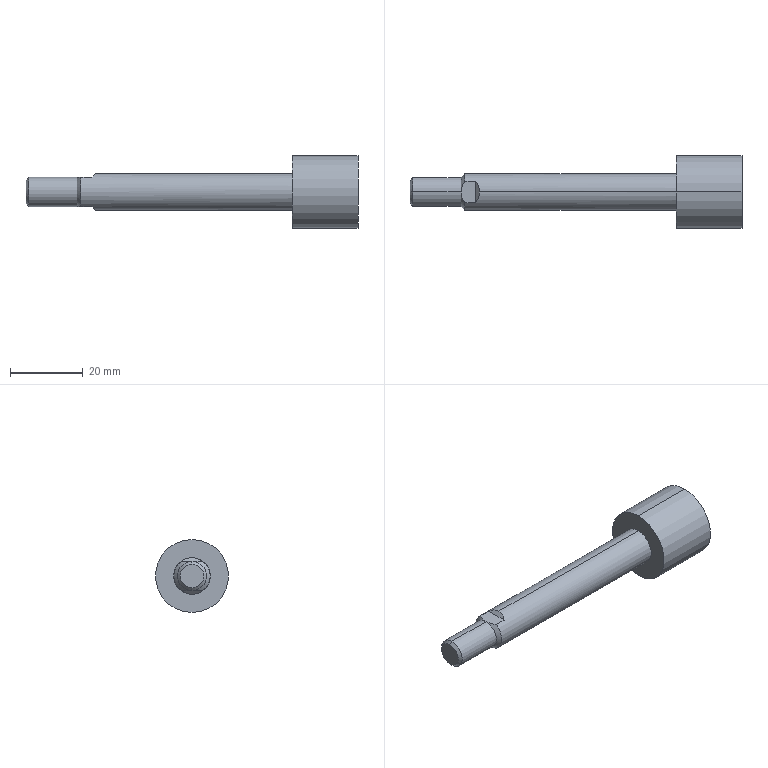Part | SolidWorks | features BaseBody 1 | 1 solid | 17 faces | box 91 x 20 x 20 mm | volume 10940 mm3 | plane 7 | cylinder 6 | cone 4 | commonest cylinder face diameters 8 x2 10 x2 20 x2
STEP:
#1=CARTESIAN_POINT('',(0.5,0.,5.));
#2=VERTEX_POINT('',#1);
#3=CARTESIAN_POINT('',(-0.5,3.,4.));
#4=VERTEX_POINT('',#3);
#5=CARTESIAN_POINT('',(0.5,0.,5.));
#6=CARTESIAN_POINT('',(0.5,1.091,5.));
#7=CARTESIAN_POINT('',(0.1549,2.127,4.655));
#8=CARTESIAN_POINT('',(-0.5,3.,4.));
#9=(BOUNDED_CURVE()B_SPLINE_CURVE(3,(#5,#6,#7,#8),.UNSPECIFIED.,.F.,.F.)B_SPLINE_CURVE_WITH_KNOTS((4,4),(0.,0.6435),.UNSPECIFIED.)CURVE()GEOMETRIC_REPRESENTATION_ITEM()RATIONAL_B_SPLINE_CURVE((1.,0.9658,0.9658,1.))REPRESENTATION_ITEM(''));
#10=EDGE_CURVE('',#2,#4,#9,.T.);
#11=ORIENTED_EDGE('',*,*,#10,.F.);
#12=CARTESIAN_POINT('',(54.5,0.,5.));
#13=VERTEX_POINT('',#12);
#14=CARTESIAN_POINT('',(72.5,0.,5.));
#15=DIRECTION('',(1.,0.,0.));
#16=VECTOR('',#15,1000.);
#17=LINE('',#14,#16);
#18=EDGE_CURVE('',#2,#13,#17,.T.);
#19=ORIENTED_EDGE('',*,*,#18,.T.);
#20=CARTESIAN_POINT('',(54.5,0.,-5.));
#21=VERTEX_POINT('',#20);
#22=CARTESIAN_POINT('',(54.5,0.,0.));
#23=DIRECTION('',(1.,0.,0.));
#24=DIRECTION('',(0.,0.,-1.));
#25=AXIS2_PLACEMENT_3D('',#22,#23,#24);
#26=CIRCLE('',#25,5.);
#27=EDGE_CURVE('',#21,#13,#26,.T.);
#28=ORIENTED_EDGE('',*,*,#27,.F.);
#29=CARTESIAN_POINT('',(0.5,0.,-5.));
#30=VERTEX_POINT('',#29);
#31=CARTESIAN_POINT('',(72.5,0.,-5.));
#32=DIRECTION('',(1.,0.,0.));
#33=VECTOR('',#32,1000.);
#34=LINE('',#31,#33);
#35=EDGE_CURVE('',#30,#21,#34,.T.);
#36=ORIENTED_EDGE('',*,*,#35,.F.);
#37=CARTESIAN_POINT('',(-0.5,3.,-4.));
#38=VERTEX_POINT('',#37);
#39=CARTESIAN_POINT('',(-0.5,3.,-4.));
#40=CARTESIAN_POINT('',(0.1549,2.127,-4.655));
#41=CARTESIAN_POINT('',(0.5,1.091,-5.));
#42=CARTESIAN_POINT('',(0.5,0.,-5.));
#43=(BOUNDED_CURVE()B_SPLINE_CURVE(3,(#39,#40,#41,#42),.UNSPECIFIED.,.F.,.T.)B_SPLINE_CURVE_WITH_KNOTS((4,4),(5.64,6.283),.UNSPECIFIED.)CURVE()GEOMETRIC_REPRESENTATION_ITEM()RATIONAL_B_SPLINE_CURVE((1.,0.9658,0.9658,1.))REPRESENTATION_ITEM(''));
#44=EDGE_CURVE('',#38,#30,#43,.T.);
#45=ORIENTED_EDGE('',*,*,#44,.F.);
#46=CARTESIAN_POINT('',(-3.5,3.,-4.));
#47=VERTEX_POINT('',#46);
#48=CARTESIAN_POINT('',(72.5,3.,-4.));
#49=DIRECTION('',(1.,0.,0.));
#50=VECTOR('',#49,1000.);
#51=LINE('',#48,#50);
#52=EDGE_CURVE('',#47,#38,#51,.T.);
#53=ORIENTED_EDGE('',*,*,#52,.F.);
#54=CARTESIAN_POINT('',(-3.5,3.,4.));
#55=VERTEX_POINT('',#54);
#56=CARTESIAN_POINT('',(-3.5,0.,0.));
#57=DIRECTION('',(1.,0.,0.));
#58=DIRECTION('',(0.,0.,-1.));
#59=AXIS2_PLACEMENT_3D('',#56,#57,#58);
#60=CIRCLE('',#59,5.);
#61=EDGE_CURVE('',#47,#55,#60,.T.);
#62=ORIENTED_EDGE('',*,*,#61,.T.);
#63=CARTESIAN_POINT('',(72.5,3.,4.));
#64=DIRECTION('',(-1.,0.,0.));
#65=VECTOR('',#64,1000.);
#66=LINE('',#63,#65);
#67=EDGE_CURVE('',#4,#55,#66,.T.);
#68=ORIENTED_EDGE('',*,*,#67,.F.);
#69=EDGE_LOOP('',(#11,#19,#28,#36,#45,#53,#62,#68));
#70=FACE_OUTER_BOUND('',#69,.T.);
#71=CARTESIAN_POINT('',(72.5,0.,0.));
#72=DIRECTION('',(1.,0.,0.));
#73=DIRECTION('',(0.,0.,-1.));
#74=AXIS2_PLACEMENT_3D('',#71,#72,#73);
#75=CYLINDRICAL_SURFACE('',#74,5.);
#76=ADVANCED_FACE('',(#70),#75,.T.);
#77=CARTESIAN_POINT('',(54.5,0.,-10.));
#78=VERTEX_POINT('',#77);
#79=CARTESIAN_POINT('',(54.5,0.,10.));
#80=VERTEX_POINT('',#79);
#81=CARTESIAN_POINT('',(54.5,0.,0.));
#82=DIRECTION('',(1.,0.,0.));
#83=DIRECTION('',(0.,0.,-1.));
#84=AXIS2_PLACEMENT_3D('',#81,#82,#83);
#85=CIRCLE('',#84,10.);
#86=EDGE_CURVE('',#78,#80,#85,.T.);
#87=ORIENTED_EDGE('',*,*,#86,.T.);
#88=CARTESIAN_POINT('',(72.5,0.,10.));
#89=VERTEX_POINT('',#88);
#90=CARTESIAN_POINT('',(72.5,0.,10.));
#91=DIRECTION('',(1.,0.,0.));
#92=VECTOR('',#91,1000.);
#93=LINE('',#90,#92);
#94=EDGE_CURVE('',#80,#89,#93,.T.);
#95=ORIENTED_EDGE('',*,*,#94,.T.);
#96=CARTESIAN_POINT('',(72.5,0.,-10.));
#97=VERTEX_POINT('',#96);
#98=CARTESIAN_POINT('',(72.5,0.,0.));
#99=DIRECTION('',(1.,0.,0.));
#100=DIRECTION('',(0.,0.,-1.));
#101=AXIS2_PLACEMENT_3D('',#98,#99,#100);
#102=CIRCLE('',#101,10.);
#103=EDGE_CURVE('',#97,#89,#102,.T.);
#104=ORIENTED_EDGE('',*,*,#103,.F.);
#105=CARTESIAN_POINT('',(72.5,0.,-10.));
#106=DIRECTION('',(1.,0.,0.));
#107=VECTOR('',#106,1000.);
#108=LINE('',#105,#107);
#109=EDGE_CURVE('',#78,#97,#108,.T.);
#110=ORIENTED_EDGE('',*,*,#109,.F.);
#111=EDGE_LOOP('',(#87,#95,#104,#110));
#112=FACE_OUTER_BOUND('',#111,.T.);
#113=CARTESIAN_POINT('',(72.5,0.,0.));
#114=DIRECTION('',(1.,0.,0.));
#115=DIRECTION('',(0.,0.,-1.));
#116=AXIS2_PLACEMENT_3D('',#113,#114,#115);
#117=CYLINDRICAL_SURFACE('',#116,10.);
#118=ADVANCED_FACE('',(#112),#117,.T.);
#119=CARTESIAN_POINT('',(-18.5,0.,-3.233));
#120=VERTEX_POINT('',#119);
#121=CARTESIAN_POINT('',(-18.5,0.,3.233));
#122=VERTEX_POINT('',#121);
#123=CARTESIAN_POINT('',(-18.5,0.,0.));
#124=DIRECTION('',(1.,0.,0.));
#125=DIRECTION('',(0.,0.,-1.));
#126=AXIS2_PLACEMENT_3D('',#123,#124,#125);
#127=CIRCLE('',#126,3.233);
#128=EDGE_CURVE('',#120,#122,#127,.T.);
#129=ORIENTED_EDGE('',*,*,#128,.T.);
#130=CARTESIAN_POINT('',(-17.733,0.,4.));
#131=VERTEX_POINT('',#130);
#132=CARTESIAN_POINT('',(-18.5,0.,3.233));
#133=DIRECTION('',(0.7071,0.,0.7071));
#134=VECTOR('',#133,1000.);
#135=LINE('',#132,#134);
#136=EDGE_CURVE('',#122,#131,#135,.T.);
#137=ORIENTED_EDGE('',*,*,#136,.T.);
#138=CARTESIAN_POINT('',(-17.733,0.,-4.));
#139=VERTEX_POINT('',#138);
#140=CARTESIAN_POINT('',(-17.733,0.,0.));
#141=DIRECTION('',(1.,0.,0.));
#142=DIRECTION('',(0.,0.,-1.));
#143=AXIS2_PLACEMENT_3D('',#140,#141,#142);
#144=CIRCLE('',#143,4.);
#145=EDGE_CURVE('',#139,#131,#144,.T.);
#146=ORIENTED_EDGE('',*,*,#145,.F.);
#147=CARTESIAN_POINT('',(-18.5,0.,-3.233));
#148=DIRECTION('',(0.7071,0.,-0.7071));
#149=VECTOR('',#148,1000.);
#150=LINE('',#147,#149);
#151=EDGE_CURVE('',#120,#139,#150,.T.);
#152=ORIENTED_EDGE('',*,*,#151,.F.);
#153=EDGE_LOOP('',(#129,#137,#146,#152));
#154=FACE_OUTER_BOUND('',#153,.T.);
#155=CARTESIAN_POINT('',(-18.5,0.,0.));
#156=DIRECTION('',(1.,0.,0.));
#157=DIRECTION('',(0.,0.,-1.));
#158=AXIS2_PLACEMENT_3D('',#155,#156,#157);
#159=CONICAL_SURFACE('',#158,3.233,0.7854);
#160=ADVANCED_FACE('',(#154),#159,.T.);
#161=ORIENTED_EDGE('',*,*,#145,.T.);
#162=CARTESIAN_POINT('',(-4.5,0.,4.));
#163=VERTEX_POINT('',#162);
#164=CARTESIAN_POINT('',(0.,0.,4.));
#165=DIRECTION('',(1.,0.,0.));
#166=VECTOR('',#165,1000.);
#167=LINE('',#164,#166);
#168=EDGE_CURVE('',#131,#163,#167,.T.);
#169=ORIENTED_EDGE('',*,*,#168,.T.);
#170=CARTESIAN_POINT('',(-4.5,0.,-4.));
#171=VERTEX_POINT('',#170);
#172=CARTESIAN_POINT('',(-4.5,0.,0.));
#173=DIRECTION('',(1.,0.,0.));
#174=DIRECTION('',(0.,0.,-1.));
#175=AXIS2_PLACEMENT_3D('',#172,#173,#174);
#176=CIRCLE('',#175,4.);
#177=EDGE_CURVE('',#171,#163,#176,.T.);
#178=ORIENTED_EDGE('',*,*,#177,.F.);
#179=CARTESIAN_POINT('',(0.,0.,-4.));
#180=DIRECTION('',(1.,0.,0.));
#181=VECTOR('',#180,1000.);
#182=LINE('',#179,#181);
#183=EDGE_CURVE('',#139,#171,#182,.T.);
#184=ORIENTED_EDGE('',*,*,#183,.F.);
#185=EDGE_LOOP('',(#161,#169,#178,#184));
#186=FACE_OUTER_BOUND('',#185,.T.);
#187=CARTESIAN_POINT('',(0.,0.,0.));
#188=DIRECTION('',(1.,0.,0.));
#189=DIRECTION('',(0.,0.,-1.));
#190=AXIS2_PLACEMENT_3D('',#187,#188,#189);
#191=CYLINDRICAL_SURFACE('',#190,4.);
#192=ADVANCED_FACE('',(#186),#191,.T.);
#193=CARTESIAN_POINT('',(-3.5,-3.,4.));
#194=VERTEX_POINT('',#193);
#195=CARTESIAN_POINT('',(-0.5,-3.,4.));
#196=VERTEX_POINT('',#195);
#197=CARTESIAN_POINT('',(72.5,-3.,4.));
#198=DIRECTION('',(1.,0.,0.));
#199=VECTOR('',#198,1000.);
#200=LINE('',#197,#199);
#201=EDGE_CURVE('',#194,#196,#200,.T.);
#202=ORIENTED_EDGE('',*,*,#201,.T.);
#203=CARTESIAN_POINT('',(-0.5,8.,4.));
#204=DIRECTION('',(0.,-1.,0.));
#205=VECTOR('',#204,1000.);
#206=LINE('',#203,#205);
#207=EDGE_CURVE('',#4,#196,#206,.T.);
#208=ORIENTED_EDGE('',*,*,#207,.F.);
#209=ORIENTED_EDGE('',*,*,#67,.T.);
#210=CARTESIAN_POINT('',(-3.5,3.,4.));
#211=CARTESIAN_POINT('',(-3.656,2.741,4.));
#212=CARTESIAN_POINT('',(-3.86,2.368,4.));
#213=CARTESIAN_POINT('',(-4.048,1.961,4.));
#214=CARTESIAN_POINT('',(-4.129,1.765,4.));
#215=CARTESIAN_POINT('',(-4.166,1.669,4.));
#216=CARTESIAN_POINT('',(-4.184,1.622,4.));
#217=CARTESIAN_POINT('',(-4.192,1.601,4.));
#218=CARTESIAN_POINT('',(-4.196,1.588,4.));
#219=CARTESIAN_POINT('',(-4.198,1.583,4.));
#220=CARTESIAN_POINT('',(-4.4,1.024,4.));
#221=CARTESIAN_POINT('',(-4.5,0.4995,4.));
#222=CARTESIAN_POINT('',(-4.5,0.,4.));
#223=B_SPLINE_CURVE_WITH_KNOTS('',3,(#210,#211,#212,#213,#214,#215,#216,#217,#218,#219,#220,#221,#222),.UNSPECIFIED.,.F.,.F.,(4,1,1,1,1,1,2,2,4),(0.,0.25,0.375,0.4375,0.4687,0.4844,0.4922,0.5,1.),.UNSPECIFIED.);
#224=EDGE_CURVE('',#55,#163,#223,.T.);
#225=ORIENTED_EDGE('',*,*,#224,.T.);
#226=CARTESIAN_POINT('',(-4.5,0.,4.));
#227=CARTESIAN_POINT('',(-4.5,-0.249,4.));
#228=CARTESIAN_POINT('',(-4.463,-0.6316,4.));
#229=CARTESIAN_POINT('',(-4.355,-1.094,4.));
#230=CARTESIAN_POINT('',(-4.285,-1.329,4.));
#231=CARTESIAN_POINT('',(-4.246,-1.447,4.));
#232=CARTESIAN_POINT('',(-4.225,-1.507,4.));
#233=CARTESIAN_POINT('',(-4.216,-1.533,4.));
#234=CARTESIAN_POINT('',(-4.21,-1.55,4.));
#235=CARTESIAN_POINT('',(-4.207,-1.56,4.));
#236=CARTESIAN_POINT('',(-4.047,-2.001,4.));
#237=CARTESIAN_POINT('',(-3.812,-2.479,4.));
#238=CARTESIAN_POINT('',(-3.5,-3.,4.));
#239=B_SPLINE_CURVE_WITH_KNOTS('',3,(#226,#227,#228,#229,#230,#231,#232,#233,#234,#235,#236,#237,#238),.UNSPECIFIED.,.F.,.F.,(4,1,1,1,1,1,2,2,4),(0.,0.25,0.375,0.4375,0.4687,0.4844,0.4922,0.5,1.),.UNSPECIFIED.);
#240=EDGE_CURVE('',#163,#194,#239,.T.);
#241=ORIENTED_EDGE('',*,*,#240,.T.);
#242=EDGE_LOOP('',(#202,#208,#209,#225,#241));
#243=FACE_OUTER_BOUND('',#242,.T.);
#244=CARTESIAN_POINT('',(-0.5,8.,4.));
#245=DIRECTION('',(0.,0.,1.));
#246=DIRECTION('',(1.,0.,0.));
#247=AXIS2_PLACEMENT_3D('',#244,#245,#246);
#248=PLANE('',#247);
#249=ADVANCED_FACE('',(#243),#248,.T.);
#250=CARTESIAN_POINT('',(-0.5,-3.,4.));
#251=CARTESIAN_POINT('',(0.1549,-2.127,4.655));
#252=CARTESIAN_POINT('',(0.5,-1.091,5.));
#253=CARTESIAN_POINT('',(0.5,0.,5.));
#254=(BOUNDED_CURVE()B_SPLINE_CURVE(3,(#250,#251,#252,#253),.UNSPECIFIED.,.F.,.T.)B_SPLINE_CURVE_WITH_KNOTS((4,4),(5.64,6.283),.UNSPECIFIED.)CURVE()GEOMETRIC_REPRESENTATION_ITEM()RATIONAL_B_SPLINE_CURVE((1.,0.9658,0.9658,1.))REPRESENTATION_ITEM(''));
#255=EDGE_CURVE('',#196,#2,#254,.T.);
#256=ORIENTED_EDGE('',*,*,#255,.T.);
#257=ORIENTED_EDGE('',*,*,#10,.T.);
#258=ORIENTED_EDGE('',*,*,#207,.T.);
#259=EDGE_LOOP('',(#256,#257,#258));
#260=FACE_OUTER_BOUND('',#259,.T.);
#261=CARTESIAN_POINT('',(19.5,8.,24.));
#262=DIRECTION('',(-0.7071,0.,0.7071));
#263=DIRECTION('',(0.,1.,0.));
#264=AXIS2_PLACEMENT_3D('',#261,#262,#263);
#265=PLANE('',#264);
#266=ADVANCED_FACE('',(#260),#265,.T.);
#267=ORIENTED_EDGE('',*,*,#44,.T.);
#268=CARTESIAN_POINT('',(-0.5,-3.,-4.));
#269=VERTEX_POINT('',#268);
#270=CARTESIAN_POINT('',(0.5,0.,-5.));
#271=CARTESIAN_POINT('',(0.5,-1.091,-5.));
#272=CARTESIAN_POINT('',(0.1549,-2.127,-4.655));
#273=CARTESIAN_POINT('',(-0.5,-3.,-4.));
#274=(BOUNDED_CURVE()B_SPLINE_CURVE(3,(#270,#271,#272,#273),.UNSPECIFIED.,.F.,.F.)B_SPLINE_CURVE_WITH_KNOTS((4,4),(0.,0.6435),.UNSPECIFIED.)CURVE()GEOMETRIC_REPRESENTATION_ITEM()RATIONAL_B_SPLINE_CURVE((1.,0.9658,0.9658,1.))REPRESENTATION_ITEM(''));
#275=EDGE_CURVE('',#30,#269,#274,.T.);
#276=ORIENTED_EDGE('',*,*,#275,.T.);
#277=CARTESIAN_POINT('',(-0.5,8.,-4.));
#278=DIRECTION('',(0.,-1.,0.));
#279=VECTOR('',#278,1000.);
#280=LINE('',#277,#279);
#281=EDGE_CURVE('',#38,#269,#280,.T.);
#282=ORIENTED_EDGE('',*,*,#281,.F.);
#283=EDGE_LOOP('',(#267,#276,#282));
#284=FACE_OUTER_BOUND('',#283,.T.);
#285=CARTESIAN_POINT('',(-0.5,8.,-4.));
#286=DIRECTION('',(-0.7071,0.,-0.7071));
#287=DIRECTION('',(-0.7071,0.,0.7071));
#288=AXIS2_PLACEMENT_3D('',#285,#286,#287);
#289=PLANE('',#288);
#290=ADVANCED_FACE('',(#284),#289,.T.);
#291=ORIENTED_EDGE('',*,*,#52,.T.);
#292=ORIENTED_EDGE('',*,*,#281,.T.);
#293=CARTESIAN_POINT('',(-3.5,-3.,-4.));
#294=VERTEX_POINT('',#293);
#295=CARTESIAN_POINT('',(72.5,-3.,-4.));
#296=DIRECTION('',(-1.,0.,0.));
#297=VECTOR('',#296,1000.);
#298=LINE('',#295,#297);
#299=EDGE_CURVE('',#269,#294,#298,.T.);
#300=ORIENTED_EDGE('',*,*,#299,.T.);
#301=CARTESIAN_POINT('',(-3.5,-3.,-4.));
#302=CARTESIAN_POINT('',(-3.656,-2.741,-4.));
#303=CARTESIAN_POINT('',(-3.86,-2.368,-4.));
#304=CARTESIAN_POINT('',(-4.048,-1.961,-4.));
#305=CARTESIAN_POINT('',(-4.129,-1.765,-4.));
#306=CARTESIAN_POINT('',(-4.166,-1.669,-4.));
#307=CARTESIAN_POINT('',(-4.184,-1.622,-4.));
#308=CARTESIAN_POINT('',(-4.192,-1.601,-4.));
#309=CARTESIAN_POINT('',(-4.196,-1.588,-4.));
#310=CARTESIAN_POINT('',(-4.198,-1.583,-4.));
#311=CARTESIAN_POINT('',(-4.4,-1.024,-4.));
#312=CARTESIAN_POINT('',(-4.5,-0.4995,-4.));
#313=CARTESIAN_POINT('',(-4.5,0.,-4.));
#314=B_SPLINE_CURVE_WITH_KNOTS('',3,(#301,#302,#303,#304,#305,#306,#307,#308,#309,#310,#311,#312,#313),.UNSPECIFIED.,.F.,.F.,(4,1,1,1,1,1,2,2,4),(0.,0.25,0.375,0.4375,0.4688,0.4844,0.4922,0.5,1.),.UNSPECIFIED.);
#315=EDGE_CURVE('',#294,#171,#314,.T.);
#316=ORIENTED_EDGE('',*,*,#315,.T.);
#317=CARTESIAN_POINT('',(-4.5,0.,-4.));
#318=CARTESIAN_POINT('',(-4.5,0.249,-4.));
#319=CARTESIAN_POINT('',(-4.463,0.6316,-4.));
#320=CARTESIAN_POINT('',(-4.355,1.094,-4.));
#321=CARTESIAN_POINT('',(-4.285,1.329,-4.));
#322=CARTESIAN_POINT('',(-4.246,1.447,-4.));
#323=CARTESIAN_POINT('',(-4.225,1.507,-4.));
#324=CARTESIAN_POINT('',(-4.216,1.533,-4.));
#325=CARTESIAN_POINT('',(-4.21,1.55,-4.));
#326=CARTESIAN_POINT('',(-4.207,1.56,-4.));
#327=CARTESIAN_POINT('',(-4.047,2.001,-4.));
#328=CARTESIAN_POINT('',(-3.812,2.479,-4.));
#329=CARTESIAN_POINT('',(-3.5,3.,-4.));
#330=B_SPLINE_CURVE_WITH_KNOTS('',3,(#317,#318,#319,#320,#321,#322,#323,#324,#325,#326,#327,#328,#329),.UNSPECIFIED.,.F.,.F.,(4,1,1,1,1,1,2,2,4),(0.,0.25,0.375,0.4375,0.4687,0.4844,0.4922,0.5,1.),.UNSPECIFIED.);
#331=EDGE_CURVE('',#171,#47,#330,.T.);
#332=ORIENTED_EDGE('',*,*,#331,.T.);
#333=EDGE_LOOP('',(#291,#292,#300,#316,#332));
#334=FACE_OUTER_BOUND('',#333,.T.);
#335=CARTESIAN_POINT('',(-4.5,8.,-4.));
#336=DIRECTION('',(0.,0.,-1.));
#337=DIRECTION('',(0.,-1.,0.));
#338=AXIS2_PLACEMENT_3D('',#335,#336,#337);
#339=PLANE('',#338);
#340=ADVANCED_FACE('',(#334),#339,.T.);
#341=ORIENTED_EDGE('',*,*,#168,.F.);
#342=CARTESIAN_POINT('',(-17.733,0.,0.));
#343=DIRECTION('',(1.,0.,0.));
#344=DIRECTION('',(0.,0.,-1.));
#345=AXIS2_PLACEMENT_3D('',#342,#343,#344);
#346=CIRCLE('',#345,4.);
#347=EDGE_CURVE('',#131,#139,#346,.T.);
#348=ORIENTED_EDGE('',*,*,#347,.T.);
#349=ORIENTED_EDGE('',*,*,#183,.T.);
#350=CARTESIAN_POINT('',(-4.5,0.,0.));
#351=DIRECTION('',(1.,0.,0.));
#352=DIRECTION('',(0.,0.,-1.));
#353=AXIS2_PLACEMENT_3D('',#350,#351,#352);
#354=CIRCLE('',#353,4.);
#355=EDGE_CURVE('',#163,#171,#354,.T.);
#356=ORIENTED_EDGE('',*,*,#355,.F.);
#357=EDGE_LOOP('',(#341,#348,#349,#356));
#358=FACE_OUTER_BOUND('',#357,.T.);
#359=CARTESIAN_POINT('',(0.,0.,0.));
#360=DIRECTION('',(1.,0.,0.));
#361=DIRECTION('',(0.,0.,-1.));
#362=AXIS2_PLACEMENT_3D('',#359,#360,#361);
#363=CYLINDRICAL_SURFACE('',#362,4.);
#364=ADVANCED_FACE('',(#358),#363,.T.);
#365=ORIENTED_EDGE('',*,*,#136,.F.);
#366=CARTESIAN_POINT('',(-18.5,0.,0.));
#367=DIRECTION('',(1.,0.,0.));
#368=DIRECTION('',(0.,0.,-1.));
#369=AXIS2_PLACEMENT_3D('',#366,#367,#368);
#370=CIRCLE('',#369,3.233);
#371=EDGE_CURVE('',#122,#120,#370,.T.);
#372=ORIENTED_EDGE('',*,*,#371,.T.);
#373=ORIENTED_EDGE('',*,*,#151,.T.);
#374=ORIENTED_EDGE('',*,*,#347,.F.);
#375=EDGE_LOOP('',(#365,#372,#373,#374));
#376=FACE_OUTER_BOUND('',#375,.T.);
#377=CARTESIAN_POINT('',(-18.5,0.,0.));
#378=DIRECTION('',(1.,0.,0.));
#379=DIRECTION('',(0.,0.,-1.));
#380=AXIS2_PLACEMENT_3D('',#377,#378,#379);
#381=CONICAL_SURFACE('',#380,3.233,0.7854);
#382=ADVANCED_FACE('',(#376),#381,.T.);
#383=ORIENTED_EDGE('',*,*,#128,.F.);
#384=ORIENTED_EDGE('',*,*,#371,.F.);
#385=EDGE_LOOP('',(#383,#384));
#386=FACE_OUTER_BOUND('',#385,.T.);
#387=CARTESIAN_POINT('',(-18.5,0.,0.));
#388=DIRECTION('',(1.,0.,0.));
#389=DIRECTION('',(0.,1.,0.));
#390=AXIS2_PLACEMENT_3D('',#387,#388,#389);
#391=PLANE('',#390);
#392=ADVANCED_FACE('',(#386),#391,.F.);
#393=ORIENTED_EDGE('',*,*,#103,.T.);
#394=CARTESIAN_POINT('',(72.5,0.,0.));
#395=DIRECTION('',(1.,0.,0.));
#396=DIRECTION('',(0.,0.,-1.));
#397=AXIS2_PLACEMENT_3D('',#394,#395,#396);
#398=CIRCLE('',#397,10.);
#399=EDGE_CURVE('',#89,#97,#398,.T.);
#400=ORIENTED_EDGE('',*,*,#399,.T.);
#401=EDGE_LOOP('',(#393,#400));
#402=FACE_OUTER_BOUND('',#401,.T.);
#403=CARTESIAN_POINT('',(72.5,10.,0.));
#404=DIRECTION('',(-1.,0.,0.));
#405=DIRECTION('',(0.,0.,1.));
#406=AXIS2_PLACEMENT_3D('',#403,#404,#405);
#407=PLANE('',#406);
#408=ADVANCED_FACE('',(#402),#407,.F.);
#409=ORIENTED_EDGE('',*,*,#94,.F.);
#410=CARTESIAN_POINT('',(54.5,0.,0.));
#411=DIRECTION('',(1.,0.,0.));
#412=DIRECTION('',(0.,0.,-1.));
#413=AXIS2_PLACEMENT_3D('',#410,#411,#412);
#414=CIRCLE('',#413,10.);
#415=EDGE_CURVE('',#80,#78,#414,.T.);
#416=ORIENTED_EDGE('',*,*,#415,.T.);
#417=ORIENTED_EDGE('',*,*,#109,.T.);
#418=ORIENTED_EDGE('',*,*,#399,.F.);
#419=EDGE_LOOP('',(#409,#416,#417,#418));
#420=FACE_OUTER_BOUND('',#419,.T.);
#421=CARTESIAN_POINT('',(72.5,0.,0.));
#422=DIRECTION('',(1.,0.,0.));
#423=DIRECTION('',(0.,0.,-1.));
#424=AXIS2_PLACEMENT_3D('',#421,#422,#423);
#425=CYLINDRICAL_SURFACE('',#424,10.);
#426=ADVANCED_FACE('',(#420),#425,.T.);
#427=ORIENTED_EDGE('',*,*,#27,.T.);
#428=CARTESIAN_POINT('',(54.5,0.,0.));
#429=DIRECTION('',(1.,0.,0.));
#430=DIRECTION('',(0.,0.,-1.));
#431=AXIS2_PLACEMENT_3D('',#428,#429,#430);
#432=CIRCLE('',#431,5.);
#433=EDGE_CURVE('',#13,#21,#432,.T.);
#434=ORIENTED_EDGE('',*,*,#433,.T.);
#435=EDGE_LOOP('',(#427,#434));
#436=FACE_BOUND('',#435,.T.);
#437=ORIENTED_EDGE('',*,*,#86,.F.);
#438=ORIENTED_EDGE('',*,*,#415,.F.);
#439=EDGE_LOOP('',(#437,#438));
#440=FACE_OUTER_BOUND('',#439,.T.);
#441=CARTESIAN_POINT('',(54.5,5.,0.));
#442=DIRECTION('',(1.,0.,0.));
#443=DIRECTION('',(0.,1.,0.));
#444=AXIS2_PLACEMENT_3D('',#441,#442,#443);
#445=PLANE('',#444);
#446=ADVANCED_FACE('',(#436,#440),#445,.F.);
#447=ORIENTED_EDGE('',*,*,#331,.F.);
#448=ORIENTED_EDGE('',*,*,#177,.T.);
#449=ORIENTED_EDGE('',*,*,#224,.F.);
#450=ORIENTED_EDGE('',*,*,#61,.F.);
#451=EDGE_LOOP('',(#447,#448,#449,#450));
#452=FACE_OUTER_BOUND('',#451,.T.);
#453=CARTESIAN_POINT('',(-4.5,0.,0.));
#454=DIRECTION('',(1.,0.,0.));
#455=DIRECTION('',(0.,0.,-1.));
#456=AXIS2_PLACEMENT_3D('',#453,#454,#455);
#457=CONICAL_SURFACE('',#456,4.,0.7854);
#458=ADVANCED_FACE('',(#452),#457,.T.);
#459=ORIENTED_EDGE('',*,*,#240,.F.);
#460=ORIENTED_EDGE('',*,*,#355,.T.);
#461=ORIENTED_EDGE('',*,*,#315,.F.);
#462=CARTESIAN_POINT('',(-3.5,0.,0.));
#463=DIRECTION('',(1.,0.,0.));
#464=DIRECTION('',(0.,0.,-1.));
#465=AXIS2_PLACEMENT_3D('',#462,#463,#464);
#466=CIRCLE('',#465,5.);
#467=EDGE_CURVE('',#194,#294,#466,.T.);
#468=ORIENTED_EDGE('',*,*,#467,.F.);
#469=EDGE_LOOP('',(#459,#460,#461,#468));
#470=FACE_OUTER_BOUND('',#469,.T.);
#471=CARTESIAN_POINT('',(-4.5,0.,0.));
#472=DIRECTION('',(1.,0.,0.));
#473=DIRECTION('',(0.,0.,-1.));
#474=AXIS2_PLACEMENT_3D('',#471,#472,#473);
#475=CONICAL_SURFACE('',#474,4.,0.7854);
#476=ADVANCED_FACE('',(#470),#475,.T.);
#477=ORIENTED_EDGE('',*,*,#18,.F.);
#478=ORIENTED_EDGE('',*,*,#255,.F.);
#479=ORIENTED_EDGE('',*,*,#201,.F.);
#480=ORIENTED_EDGE('',*,*,#467,.T.);
#481=ORIENTED_EDGE('',*,*,#299,.F.);
#482=ORIENTED_EDGE('',*,*,#275,.F.);
#483=ORIENTED_EDGE('',*,*,#35,.T.);
#484=ORIENTED_EDGE('',*,*,#433,.F.);
#485=EDGE_LOOP('',(#477,#478,#479,#480,#481,#482,#483,#484));
#486=FACE_OUTER_BOUND('',#485,.T.);
#487=CARTESIAN_POINT('',(72.5,0.,0.));
#488=DIRECTION('',(1.,0.,0.));
#489=DIRECTION('',(0.,0.,-1.));
#490=AXIS2_PLACEMENT_3D('',#487,#488,#489);
#491=CYLINDRICAL_SURFACE('',#490,5.);
#492=ADVANCED_FACE('',(#486),#491,.T.);
#493=CLOSED_SHELL('',(#76,#118,#160,#192,#249,#266,#290,#340,#364,#382,#392,#408,#426,#446,#458,#476,#492));
#494=MANIFOLD_SOLID_BREP('',#493);
#495=CARTESIAN_POINT('',(0.,0.,0.));
#496=DIRECTION('',(0.,0.,1.));
#497=DIRECTION('',(1.,0.,0.));
#498=AXIS2_PLACEMENT_3D('',#495,#496,#497);
#499=(LENGTH_UNIT()NAMED_UNIT(*)SI_UNIT(.MILLI.,.METRE.));
#500=UNCERTAINTY_MEASURE_WITH_UNIT(LENGTH_MEASURE(0.00001),#499,'','');
#501=(NAMED_UNIT(*)PLANE_ANGLE_UNIT()SI_UNIT($,.RADIAN.));
#502=(NAMED_UNIT(*)SI_UNIT($,.STERADIAN.)SOLID_ANGLE_UNIT());
#503=(GEOMETRIC_REPRESENTATION_CONTEXT(3)GLOBAL_UNCERTAINTY_ASSIGNED_CONTEXT((#500))GLOBAL_UNIT_ASSIGNED_CONTEXT((#499,#501,#502))REPRESENTATION_CONTEXT('',''));
#504=ADVANCED_BREP_SHAPE_REPRESENTATION('',(#494,#498),#503);